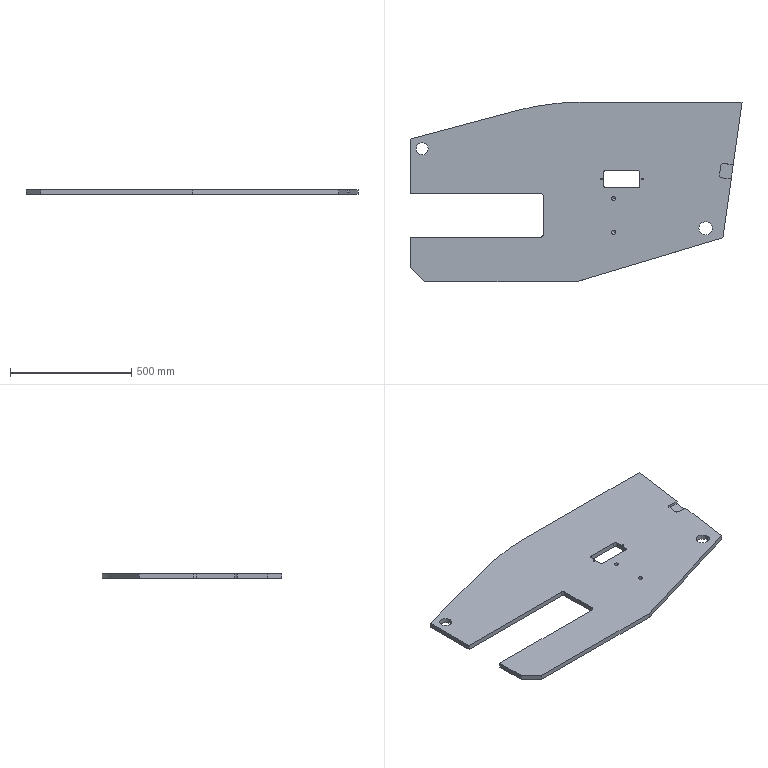Part | SolidWorks | features HoleWzd 2, FlatPattern 1, ICE 1, SMBaseFlange 1, SheetMetal 1 | 1 solid | 50 faces | box 1372 x 742.1 x 20 mm | volume 15301514 mm3 | cylinder 21 | plane 21 | cone 8 | commonest cylinder face diameters 20 x8 6.8 x4 17.5 x4 50 x2 55 x2 2000 x1
STEP:
#1=CARTESIAN_POINT('',(833.25,344.5,-12.));
#2=VERTEX_POINT('',#1);
#3=CARTESIAN_POINT('',(850.75,344.5,-12.));
#4=VERTEX_POINT('',#3);
#5=CARTESIAN_POINT('',(842.,344.5,-12.));
#6=DIRECTION('',(0.,0.,1.));
#7=DIRECTION('',(1.,0.,0.));
#8=AXIS2_PLACEMENT_3D('',#5,#6,#7);
#9=CIRCLE('',#8,8.75);
#10=EDGE_CURVE('',#2,#4,#9,.T.);
#11=ORIENTED_EDGE('',*,*,#10,.F.);
#12=CARTESIAN_POINT('',(833.25,344.5,0.));
#13=VERTEX_POINT('',#12);
#14=CARTESIAN_POINT('',(833.25,344.5,0.));
#15=DIRECTION('',(0.,0.,1.));
#16=VECTOR('',#15,1000.);
#17=LINE('',#14,#16);
#18=EDGE_CURVE('',#2,#13,#17,.T.);
#19=ORIENTED_EDGE('',*,*,#18,.T.);
#20=CARTESIAN_POINT('',(850.75,344.5,0.));
#21=VERTEX_POINT('',#20);
#22=CARTESIAN_POINT('',(842.,344.5,0.));
#23=DIRECTION('',(0.,0.,1.));
#24=DIRECTION('',(1.,0.,0.));
#25=AXIS2_PLACEMENT_3D('',#22,#23,#24);
#26=CIRCLE('',#25,8.75);
#27=EDGE_CURVE('',#13,#21,#26,.T.);
#28=ORIENTED_EDGE('',*,*,#27,.T.);
#29=CARTESIAN_POINT('',(850.75,344.5,0.));
#30=DIRECTION('',(0.,0.,1.));
#31=VECTOR('',#30,1000.);
#32=LINE('',#29,#31);
#33=EDGE_CURVE('',#4,#21,#32,.T.);
#34=ORIENTED_EDGE('',*,*,#33,.F.);
#35=EDGE_LOOP('',(#11,#19,#28,#34));
#36=FACE_OUTER_BOUND('',#35,.T.);
#37=CARTESIAN_POINT('',(842.,344.5,0.));
#38=DIRECTION('',(0.,0.,1.));
#39=DIRECTION('',(1.,0.,0.));
#40=AXIS2_PLACEMENT_3D('',#37,#38,#39);
#41=CYLINDRICAL_SURFACE('',#40,8.75);
#42=ADVANCED_FACE('',(#36),#41,.F.);
#43=CARTESIAN_POINT('',(842.,344.5,-17.258));
#44=VERTEX_POINT('',#43);
#45=CARTESIAN_POINT('',(850.75,344.5,-12.));
#46=DIRECTION('',(0.8572,0.,0.515));
#47=VECTOR('',#46,1000.);
#48=LINE('',#45,#47);
#49=EDGE_CURVE('',#44,#4,#48,.T.);
#50=ORIENTED_EDGE('',*,*,#49,.F.);
#51=CARTESIAN_POINT('',(833.25,344.5,-12.));
#52=DIRECTION('',(-0.8572,0.,0.515));
#53=VECTOR('',#52,1000.);
#54=LINE('',#51,#53);
#55=EDGE_CURVE('',#44,#2,#54,.T.);
#56=ORIENTED_EDGE('',*,*,#55,.T.);
#57=ORIENTED_EDGE('',*,*,#10,.T.);
#58=EDGE_LOOP('',(#50,#56,#57));
#59=FACE_OUTER_BOUND('',#58,.T.);
#60=CARTESIAN_POINT('',(842.,344.5,-12.));
#61=DIRECTION('',(0.,0.,1.));
#62=DIRECTION('',(1.,0.,0.));
#63=AXIS2_PLACEMENT_3D('',#60,#61,#62);
#64=CONICAL_SURFACE('',#63,8.75,1.03);
#65=ADVANCED_FACE('',(#59),#64,.F.);
#66=CARTESIAN_POINT('',(833.25,204.5,-12.));
#67=VERTEX_POINT('',#66);
#68=CARTESIAN_POINT('',(850.75,204.5,-12.));
#69=VERTEX_POINT('',#68);
#70=CARTESIAN_POINT('',(842.,204.5,-12.));
#71=DIRECTION('',(0.,0.,1.));
#72=DIRECTION('',(1.,0.,0.));
#73=AXIS2_PLACEMENT_3D('',#70,#71,#72);
#74=CIRCLE('',#73,8.75);
#75=EDGE_CURVE('',#67,#69,#74,.T.);
#76=ORIENTED_EDGE('',*,*,#75,.F.);
#77=CARTESIAN_POINT('',(833.25,204.5,0.));
#78=VERTEX_POINT('',#77);
#79=CARTESIAN_POINT('',(833.25,204.5,0.));
#80=DIRECTION('',(0.,0.,1.));
#81=VECTOR('',#80,1000.);
#82=LINE('',#79,#81);
#83=EDGE_CURVE('',#67,#78,#82,.T.);
#84=ORIENTED_EDGE('',*,*,#83,.T.);
#85=CARTESIAN_POINT('',(850.75,204.5,0.));
#86=VERTEX_POINT('',#85);
#87=CARTESIAN_POINT('',(842.,204.5,0.));
#88=DIRECTION('',(0.,0.,1.));
#89=DIRECTION('',(1.,0.,0.));
#90=AXIS2_PLACEMENT_3D('',#87,#88,#89);
#91=CIRCLE('',#90,8.75);
#92=EDGE_CURVE('',#78,#86,#91,.T.);
#93=ORIENTED_EDGE('',*,*,#92,.T.);
#94=CARTESIAN_POINT('',(850.75,204.5,0.));
#95=DIRECTION('',(0.,0.,1.));
#96=VECTOR('',#95,1000.);
#97=LINE('',#94,#96);
#98=EDGE_CURVE('',#69,#86,#97,.T.);
#99=ORIENTED_EDGE('',*,*,#98,.F.);
#100=EDGE_LOOP('',(#76,#84,#93,#99));
#101=FACE_OUTER_BOUND('',#100,.T.);
#102=CARTESIAN_POINT('',(842.,204.5,0.));
#103=DIRECTION('',(0.,0.,1.));
#104=DIRECTION('',(1.,0.,0.));
#105=AXIS2_PLACEMENT_3D('',#102,#103,#104);
#106=CYLINDRICAL_SURFACE('',#105,8.75);
#107=ADVANCED_FACE('',(#101),#106,.F.);
#108=CARTESIAN_POINT('',(842.,204.5,-17.258));
#109=VERTEX_POINT('',#108);
#110=CARTESIAN_POINT('',(850.75,204.5,-12.));
#111=DIRECTION('',(0.8572,0.,0.515));
#112=VECTOR('',#111,1000.);
#113=LINE('',#110,#112);
#114=EDGE_CURVE('',#109,#69,#113,.T.);
#115=ORIENTED_EDGE('',*,*,#114,.F.);
#116=CARTESIAN_POINT('',(833.25,204.5,-12.));
#117=DIRECTION('',(-0.8572,0.,0.515));
#118=VECTOR('',#117,1000.);
#119=LINE('',#116,#118);
#120=EDGE_CURVE('',#109,#67,#119,.T.);
#121=ORIENTED_EDGE('',*,*,#120,.T.);
#122=ORIENTED_EDGE('',*,*,#75,.T.);
#123=EDGE_LOOP('',(#115,#121,#122));
#124=FACE_OUTER_BOUND('',#123,.T.);
#125=CARTESIAN_POINT('',(842.,204.5,-12.));
#126=DIRECTION('',(0.,0.,1.));
#127=DIRECTION('',(1.,0.,0.));
#128=AXIS2_PLACEMENT_3D('',#125,#126,#127);
#129=CONICAL_SURFACE('',#128,8.75,1.03);
#130=ADVANCED_FACE('',(#124),#129,.F.);
#131=CARTESIAN_POINT('',(786.6,424.5,-12.));
#132=VERTEX_POINT('',#131);
#133=CARTESIAN_POINT('',(793.4,424.5,-12.));
#134=VERTEX_POINT('',#133);
#135=CARTESIAN_POINT('',(790.,424.5,-12.));
#136=DIRECTION('',(0.,0.,1.));
#137=DIRECTION('',(1.,0.,0.));
#138=AXIS2_PLACEMENT_3D('',#135,#136,#137);
#139=CIRCLE('',#138,3.4);
#140=EDGE_CURVE('',#132,#134,#139,.T.);
#141=ORIENTED_EDGE('',*,*,#140,.F.);
#142=CARTESIAN_POINT('',(786.6,424.5,0.));
#143=VERTEX_POINT('',#142);
#144=CARTESIAN_POINT('',(786.6,424.5,0.));
#145=DIRECTION('',(0.,0.,1.));
#146=VECTOR('',#145,1000.);
#147=LINE('',#144,#146);
#148=EDGE_CURVE('',#132,#143,#147,.T.);
#149=ORIENTED_EDGE('',*,*,#148,.T.);
#150=CARTESIAN_POINT('',(793.4,424.5,0.));
#151=VERTEX_POINT('',#150);
#152=CARTESIAN_POINT('',(790.,424.5,0.));
#153=DIRECTION('',(0.,0.,1.));
#154=DIRECTION('',(1.,0.,0.));
#155=AXIS2_PLACEMENT_3D('',#152,#153,#154);
#156=CIRCLE('',#155,3.4);
#157=EDGE_CURVE('',#143,#151,#156,.T.);
#158=ORIENTED_EDGE('',*,*,#157,.T.);
#159=CARTESIAN_POINT('',(793.4,424.5,0.));
#160=DIRECTION('',(0.,0.,1.));
#161=VECTOR('',#160,1000.);
#162=LINE('',#159,#161);
#163=EDGE_CURVE('',#134,#151,#162,.T.);
#164=ORIENTED_EDGE('',*,*,#163,.F.);
#165=EDGE_LOOP('',(#141,#149,#158,#164));
#166=FACE_OUTER_BOUND('',#165,.T.);
#167=CARTESIAN_POINT('',(790.,424.5,0.));
#168=DIRECTION('',(0.,0.,1.));
#169=DIRECTION('',(1.,0.,0.));
#170=AXIS2_PLACEMENT_3D('',#167,#168,#169);
#171=CYLINDRICAL_SURFACE('',#170,3.4);
#172=ADVANCED_FACE('',(#166),#171,.F.);
#173=CARTESIAN_POINT('',(790.,424.5,-14.043));
#174=VERTEX_POINT('',#173);
#175=CARTESIAN_POINT('',(793.4,424.5,-12.));
#176=DIRECTION('',(0.8572,0.,0.515));
#177=VECTOR('',#176,1000.);
#178=LINE('',#175,#177);
#179=EDGE_CURVE('',#174,#134,#178,.T.);
#180=ORIENTED_EDGE('',*,*,#179,.F.);
#181=CARTESIAN_POINT('',(786.6,424.5,-12.));
#182=DIRECTION('',(-0.8572,0.,0.515));
#183=VECTOR('',#182,1000.);
#184=LINE('',#181,#183);
#185=EDGE_CURVE('',#174,#132,#184,.T.);
#186=ORIENTED_EDGE('',*,*,#185,.T.);
#187=ORIENTED_EDGE('',*,*,#140,.T.);
#188=EDGE_LOOP('',(#180,#186,#187));
#189=FACE_OUTER_BOUND('',#188,.T.);
#190=CARTESIAN_POINT('',(790.,424.5,-12.));
#191=DIRECTION('',(0.,0.,1.));
#192=DIRECTION('',(1.,0.,0.));
#193=AXIS2_PLACEMENT_3D('',#190,#191,#192);
#194=CONICAL_SURFACE('',#193,3.4,1.03);
#195=ADVANCED_FACE('',(#189),#194,.F.);
#196=CARTESIAN_POINT('',(956.6,424.5,-12.));
#197=VERTEX_POINT('',#196);
#198=CARTESIAN_POINT('',(963.4,424.5,-12.));
#199=VERTEX_POINT('',#198);
#200=CARTESIAN_POINT('',(960.,424.5,-12.));
#201=DIRECTION('',(0.,0.,1.));
#202=DIRECTION('',(1.,0.,0.));
#203=AXIS2_PLACEMENT_3D('',#200,#201,#202);
#204=CIRCLE('',#203,3.4);
#205=EDGE_CURVE('',#197,#199,#204,.T.);
#206=ORIENTED_EDGE('',*,*,#205,.F.);
#207=CARTESIAN_POINT('',(956.6,424.5,0.));
#208=VERTEX_POINT('',#207);
#209=CARTESIAN_POINT('',(956.6,424.5,0.));
#210=DIRECTION('',(0.,0.,1.));
#211=VECTOR('',#210,1000.);
#212=LINE('',#209,#211);
#213=EDGE_CURVE('',#197,#208,#212,.T.);
#214=ORIENTED_EDGE('',*,*,#213,.T.);
#215=CARTESIAN_POINT('',(963.4,424.5,0.));
#216=VERTEX_POINT('',#215);
#217=CARTESIAN_POINT('',(960.,424.5,0.));
#218=DIRECTION('',(0.,0.,1.));
#219=DIRECTION('',(1.,0.,0.));
#220=AXIS2_PLACEMENT_3D('',#217,#218,#219);
#221=CIRCLE('',#220,3.4);
#222=EDGE_CURVE('',#208,#216,#221,.T.);
#223=ORIENTED_EDGE('',*,*,#222,.T.);
#224=CARTESIAN_POINT('',(963.4,424.5,0.));
#225=DIRECTION('',(0.,0.,1.));
#226=VECTOR('',#225,1000.);
#227=LINE('',#224,#226);
#228=EDGE_CURVE('',#199,#216,#227,.T.);
#229=ORIENTED_EDGE('',*,*,#228,.F.);
#230=EDGE_LOOP('',(#206,#214,#223,#229));
#231=FACE_OUTER_BOUND('',#230,.T.);
#232=CARTESIAN_POINT('',(960.,424.5,0.));
#233=DIRECTION('',(0.,0.,1.));
#234=DIRECTION('',(1.,0.,0.));
#235=AXIS2_PLACEMENT_3D('',#232,#233,#234);
#236=CYLINDRICAL_SURFACE('',#235,3.4);
#237=ADVANCED_FACE('',(#231),#236,.F.);
#238=CARTESIAN_POINT('',(960.,424.5,-14.043));
#239=VERTEX_POINT('',#238);
#240=CARTESIAN_POINT('',(963.4,424.5,-12.));
#241=DIRECTION('',(0.8572,0.,0.515));
#242=VECTOR('',#241,1000.);
#243=LINE('',#240,#242);
#244=EDGE_CURVE('',#239,#199,#243,.T.);
#245=ORIENTED_EDGE('',*,*,#244,.F.);
#246=CARTESIAN_POINT('',(956.6,424.5,-12.));
#247=DIRECTION('',(-0.8572,0.,0.515));
#248=VECTOR('',#247,1000.);
#249=LINE('',#246,#248);
#250=EDGE_CURVE('',#239,#197,#249,.T.);
#251=ORIENTED_EDGE('',*,*,#250,.T.);
#252=ORIENTED_EDGE('',*,*,#205,.T.);
#253=EDGE_LOOP('',(#245,#251,#252));
#254=FACE_OUTER_BOUND('',#253,.T.);
#255=CARTESIAN_POINT('',(960.,424.5,-12.));
#256=DIRECTION('',(0.,0.,1.));
#257=DIRECTION('',(1.,0.,0.));
#258=AXIS2_PLACEMENT_3D('',#255,#256,#257);
#259=CONICAL_SURFACE('',#258,3.4,1.03);
#260=ADVANCED_FACE('',(#254),#259,.F.);
#261=CARTESIAN_POINT('',(1194.,220.7,-20.));
#262=VERTEX_POINT('',#261);
#263=CARTESIAN_POINT('',(1249.,220.7,-20.));
#264=VERTEX_POINT('',#263);
#265=CARTESIAN_POINT('',(1221.5,220.7,-20.));
#266=DIRECTION('',(0.,0.,1.));
#267=DIRECTION('',(1.,0.,0.));
#268=AXIS2_PLACEMENT_3D('',#265,#266,#267);
#269=CIRCLE('',#268,27.5);
#270=EDGE_CURVE('',#262,#264,#269,.T.);
#271=ORIENTED_EDGE('',*,*,#270,.F.);
#272=CARTESIAN_POINT('',(1194.,220.7,0.));
#273=VERTEX_POINT('',#272);
#274=CARTESIAN_POINT('',(1194.,220.7,-20.));
#275=DIRECTION('',(0.,0.,1.));
#276=VECTOR('',#275,1000.);
#277=LINE('',#274,#276);
#278=EDGE_CURVE('',#262,#273,#277,.T.);
#279=ORIENTED_EDGE('',*,*,#278,.T.);
#280=CARTESIAN_POINT('',(1249.,220.7,0.));
#281=VERTEX_POINT('',#280);
#282=CARTESIAN_POINT('',(1221.5,220.7,0.));
#283=DIRECTION('',(0.,0.,1.));
#284=DIRECTION('',(1.,0.,0.));
#285=AXIS2_PLACEMENT_3D('',#282,#283,#284);
#286=CIRCLE('',#285,27.5);
#287=EDGE_CURVE('',#273,#281,#286,.T.);
#288=ORIENTED_EDGE('',*,*,#287,.T.);
#289=CARTESIAN_POINT('',(1249.,220.7,-20.));
#290=DIRECTION('',(0.,0.,1.));
#291=VECTOR('',#290,1000.);
#292=LINE('',#289,#291);
#293=EDGE_CURVE('',#264,#281,#292,.T.);
#294=ORIENTED_EDGE('',*,*,#293,.F.);
#295=EDGE_LOOP('',(#271,#279,#288,#294));
#296=FACE_OUTER_BOUND('',#295,.T.);
#297=CARTESIAN_POINT('',(1221.5,220.7,-20.));
#298=DIRECTION('',(0.,0.,1.));
#299=DIRECTION('',(1.,0.,0.));
#300=AXIS2_PLACEMENT_3D('',#297,#298,#299);
#301=CYLINDRICAL_SURFACE('',#300,27.5);
#302=ADVANCED_FACE('',(#296),#301,.F.);
#303=CARTESIAN_POINT('',(25.,550.,-20.));
#304=VERTEX_POINT('',#303);
#305=CARTESIAN_POINT('',(75.,550.,-20.));
#306=VERTEX_POINT('',#305);
#307=CARTESIAN_POINT('',(50.,550.,-20.));
#308=DIRECTION('',(0.,0.,1.));
#309=DIRECTION('',(1.,0.,0.));
#310=AXIS2_PLACEMENT_3D('',#307,#308,#309);
#311=CIRCLE('',#310,25.);
#312=EDGE_CURVE('',#304,#306,#311,.T.);
#313=ORIENTED_EDGE('',*,*,#312,.F.);
#314=CARTESIAN_POINT('',(25.,550.,0.));
#315=VERTEX_POINT('',#314);
#316=CARTESIAN_POINT('',(25.,550.,-20.));
#317=DIRECTION('',(0.,0.,1.));
#318=VECTOR('',#317,1000.);
#319=LINE('',#316,#318);
#320=EDGE_CURVE('',#304,#315,#319,.T.);
#321=ORIENTED_EDGE('',*,*,#320,.T.);
#322=CARTESIAN_POINT('',(75.,550.,0.));
#323=VERTEX_POINT('',#322);
#324=CARTESIAN_POINT('',(50.,550.,0.));
#325=DIRECTION('',(0.,0.,1.));
#326=DIRECTION('',(1.,0.,0.));
#327=AXIS2_PLACEMENT_3D('',#324,#325,#326);
#328=CIRCLE('',#327,25.);
#329=EDGE_CURVE('',#315,#323,#328,.T.);
#330=ORIENTED_EDGE('',*,*,#329,.T.);
#331=CARTESIAN_POINT('',(75.,550.,-20.));
#332=DIRECTION('',(0.,0.,1.));
#333=VECTOR('',#332,1000.);
#334=LINE('',#331,#333);
#335=EDGE_CURVE('',#306,#323,#334,.T.);
#336=ORIENTED_EDGE('',*,*,#335,.F.);
#337=EDGE_LOOP('',(#313,#321,#330,#336));
#338=FACE_OUTER_BOUND('',#337,.T.);
#339=CARTESIAN_POINT('',(50.,550.,-20.));
#340=DIRECTION('',(0.,0.,1.));
#341=DIRECTION('',(1.,0.,0.));
#342=AXIS2_PLACEMENT_3D('',#339,#340,#341);
#343=CYLINDRICAL_SURFACE('',#342,25.);
#344=ADVANCED_FACE('',(#338),#343,.F.);
#345=CARTESIAN_POINT('',(0.,590.,0.));
#346=VERTEX_POINT('',#345);
#347=CARTESIAN_POINT('',(0.,364.5,0.));
#348=VERTEX_POINT('',#347);
#349=CARTESIAN_POINT('',(0.,364.5,0.));
#350=DIRECTION('',(0.,-1.,0.));
#351=VECTOR('',#350,1000.);
#352=LINE('',#349,#351);
#353=EDGE_CURVE('',#346,#348,#352,.T.);
#354=ORIENTED_EDGE('',*,*,#353,.F.);
#355=CARTESIAN_POINT('',(0.,590.,-20.));
#356=VERTEX_POINT('',#355);
#357=CARTESIAN_POINT('',(0.,590.,-20.));
#358=DIRECTION('',(0.,0.,1.));
#359=VECTOR('',#358,1000.);
#360=LINE('',#357,#359);
#361=EDGE_CURVE('',#356,#346,#360,.T.);
#362=ORIENTED_EDGE('',*,*,#361,.F.);
#363=CARTESIAN_POINT('',(0.,364.5,-20.));
#364=VERTEX_POINT('',#363);
#365=CARTESIAN_POINT('',(0.,364.5,-20.));
#366=DIRECTION('',(0.,-1.,0.));
#367=VECTOR('',#366,1000.);
#368=LINE('',#365,#367);
#369=EDGE_CURVE('',#356,#364,#368,.T.);
#370=ORIENTED_EDGE('',*,*,#369,.T.);
#371=CARTESIAN_POINT('',(0.,364.5,-20.));
#372=DIRECTION('',(0.,0.,1.));
#373=VECTOR('',#372,1000.);
#374=LINE('',#371,#373);
#375=EDGE_CURVE('',#364,#348,#374,.T.);
#376=ORIENTED_EDGE('',*,*,#375,.T.);
#377=EDGE_LOOP('',(#354,#362,#370,#376));
#378=FACE_OUTER_BOUND('',#377,.T.);
#379=CARTESIAN_POINT('',(0.,364.5,-20.));
#380=DIRECTION('',(-1.,0.,0.));
#381=DIRECTION('',(0.,0.,1.));
#382=AXIS2_PLACEMENT_3D('',#379,#380,#381);
#383=PLANE('',#382);
#384=ADVANCED_FACE('',(#378),#383,.T.);
#385=CARTESIAN_POINT('',(445.345,708.483,0.));
#386=VERTEX_POINT('',#385);
#387=CARTESIAN_POINT('',(0.,590.,0.));
#388=DIRECTION('',(-0.9664,-0.2571,0.));
#389=VECTOR('',#388,1000.);
#390=LINE('',#387,#389);
#391=EDGE_CURVE('',#386,#346,#390,.T.);
#392=ORIENTED_EDGE('',*,*,#391,.F.);
#393=CARTESIAN_POINT('',(445.345,708.483,-20.));
#394=VERTEX_POINT('',#393);
#395=CARTESIAN_POINT('',(445.345,708.483,-20.));
#396=DIRECTION('',(0.,0.,1.));
#397=VECTOR('',#396,1000.);
#398=LINE('',#395,#397);
#399=EDGE_CURVE('',#394,#386,#398,.T.);
#400=ORIENTED_EDGE('',*,*,#399,.F.);
#401=CARTESIAN_POINT('',(0.,590.,-20.));
#402=DIRECTION('',(-0.9664,-0.2571,0.));
#403=VECTOR('',#402,1000.);
#404=LINE('',#401,#403);
#405=EDGE_CURVE('',#394,#356,#404,.T.);
#406=ORIENTED_EDGE('',*,*,#405,.T.);
#407=ORIENTED_EDGE('',*,*,#361,.T.);
#408=EDGE_LOOP('',(#392,#400,#406,#407));
#409=FACE_OUTER_BOUND('',#408,.T.);
#410=CARTESIAN_POINT('',(0.,590.,-20.));
#411=DIRECTION('',(-0.2571,0.9664,0.));
#412=DIRECTION('',(-0.9664,-0.2571,0.));
#413=AXIS2_PLACEMENT_3D('',#410,#411,#412);
#414=PLANE('',#413);
#415=ADVANCED_FACE('',(#409),#414,.T.);
#416=CARTESIAN_POINT('',(702.45,742.1,0.));
#417=VERTEX_POINT('',#416);
#418=CARTESIAN_POINT('',(702.45,-257.9,0.));
#419=DIRECTION('',(0.,0.,1.));
#420=DIRECTION('',(1.,0.,0.));
#421=AXIS2_PLACEMENT_3D('',#418,#419,#420);
#422=CIRCLE('',#421,1000.);
#423=EDGE_CURVE('',#417,#386,#422,.T.);
#424=ORIENTED_EDGE('',*,*,#423,.F.);
#425=CARTESIAN_POINT('',(702.45,742.1,-20.));
#426=VERTEX_POINT('',#425);
#427=CARTESIAN_POINT('',(702.45,742.1,-20.));
#428=DIRECTION('',(0.,0.,1.));
#429=VECTOR('',#428,1000.);
#430=LINE('',#427,#429);
#431=EDGE_CURVE('',#426,#417,#430,.T.);
#432=ORIENTED_EDGE('',*,*,#431,.F.);
#433=CARTESIAN_POINT('',(702.45,-257.9,-20.));
#434=DIRECTION('',(0.,0.,1.));
#435=DIRECTION('',(1.,0.,0.));
#436=AXIS2_PLACEMENT_3D('',#433,#434,#435);
#437=CIRCLE('',#436,1000.);
#438=EDGE_CURVE('',#426,#394,#437,.T.);
#439=ORIENTED_EDGE('',*,*,#438,.T.);
#440=ORIENTED_EDGE('',*,*,#399,.T.);
#441=EDGE_LOOP('',(#424,#432,#439,#440));
#442=FACE_OUTER_BOUND('',#441,.T.);
#443=CARTESIAN_POINT('',(702.45,-257.9,-20.));
#444=DIRECTION('',(0.,0.,1.));
#445=DIRECTION('',(1.,0.,0.));
#446=AXIS2_PLACEMENT_3D('',#443,#444,#445);
#447=CYLINDRICAL_SURFACE('',#446,1000.);
#448=ADVANCED_FACE('',(#442),#447,.T.);
#449=CARTESIAN_POINT('',(1371.7,742.1,0.));
#450=VERTEX_POINT('',#449);
#451=CARTESIAN_POINT('',(702.45,742.1,0.));
#452=DIRECTION('',(-1.,0.,0.));
#453=VECTOR('',#452,1000.);
#454=LINE('',#451,#453);
#455=EDGE_CURVE('',#450,#417,#454,.T.);
#456=ORIENTED_EDGE('',*,*,#455,.F.);
#457=CARTESIAN_POINT('',(1371.7,742.1,-20.));
#458=VERTEX_POINT('',#457);
#459=CARTESIAN_POINT('',(1371.7,742.1,-20.));
#460=DIRECTION('',(0.,0.,1.));
#461=VECTOR('',#460,1000.);
#462=LINE('',#459,#461);
#463=EDGE_CURVE('',#458,#450,#462,.T.);
#464=ORIENTED_EDGE('',*,*,#463,.F.);
#465=CARTESIAN_POINT('',(702.45,742.1,-20.));
#466=DIRECTION('',(-1.,0.,0.));
#467=VECTOR('',#466,1000.);
#468=LINE('',#465,#467);
#469=EDGE_CURVE('',#458,#426,#468,.T.);
#470=ORIENTED_EDGE('',*,*,#469,.T.);
#471=ORIENTED_EDGE('',*,*,#431,.T.);
#472=EDGE_LOOP('',(#456,#464,#470,#471));
#473=FACE_OUTER_BOUND('',#472,.T.);
#474=CARTESIAN_POINT('',(702.45,742.1,-20.));
#475=DIRECTION('',(0.,1.,0.));
#476=DIRECTION('',(0.,0.,1.));
#477=AXIS2_PLACEMENT_3D('',#474,#475,#476);
#478=PLANE('',#477);
#479=ADVANCED_FACE('',(#473),#478,.T.);
#480=CARTESIAN_POINT('',(1327.066,424.218,-10.));
#481=VERTEX_POINT('',#480);
#482=CARTESIAN_POINT('',(1327.066,424.218,0.));
#483=VERTEX_POINT('',#482);
#484=CARTESIAN_POINT('',(1327.066,424.218,-10.));
#485=DIRECTION('',(0.,0.,1.));
#486=VECTOR('',#485,1000.);
#487=LINE('',#484,#486);
#488=EDGE_CURVE('',#481,#483,#487,.T.);
#489=ORIENTED_EDGE('',*,*,#488,.T.);
#490=CARTESIAN_POINT('',(1293.,181.6,0.));
#491=VERTEX_POINT('',#490);
#492=CARTESIAN_POINT('',(1371.7,742.1,0.));
#493=DIRECTION('',(0.139,0.9903,0.));
#494=VECTOR('',#493,1000.);
#495=LINE('',#492,#494);
#496=EDGE_CURVE('',#491,#483,#495,.T.);
#497=ORIENTED_EDGE('',*,*,#496,.F.);
#498=CARTESIAN_POINT('',(1293.,181.6,-20.));
#499=VERTEX_POINT('',#498);
#500=CARTESIAN_POINT('',(1293.,181.6,-20.));
#501=DIRECTION('',(0.,0.,1.));
#502=VECTOR('',#501,1000.);
#503=LINE('',#500,#502);
#504=EDGE_CURVE('',#499,#491,#503,.T.);
#505=ORIENTED_EDGE('',*,*,#504,.F.);
#506=CARTESIAN_POINT('',(1371.7,742.1,-20.));
#507=DIRECTION('',(0.139,0.9903,0.));
#508=VECTOR('',#507,1000.);
#509=LINE('',#506,#508);
#510=EDGE_CURVE('',#499,#458,#509,.T.);
#511=ORIENTED_EDGE('',*,*,#510,.T.);
#512=ORIENTED_EDGE('',*,*,#463,.T.);
#513=CARTESIAN_POINT('',(1335.409,483.635,0.));
#514=VERTEX_POINT('',#513);
#515=CARTESIAN_POINT('',(1371.7,742.1,0.));
#516=DIRECTION('',(0.139,0.9903,0.));
#517=VECTOR('',#516,1000.);
#518=LINE('',#515,#517);
#519=EDGE_CURVE('',#514,#450,#518,.T.);
#520=ORIENTED_EDGE('',*,*,#519,.F.);
#521=CARTESIAN_POINT('',(1335.409,483.635,-10.));
#522=VERTEX_POINT('',#521);
#523=CARTESIAN_POINT('',(1335.409,483.635,-10.));
#524=DIRECTION('',(0.,0.,1.));
#525=VECTOR('',#524,1000.);
#526=LINE('',#523,#525);
#527=EDGE_CURVE('',#522,#514,#526,.T.);
#528=ORIENTED_EDGE('',*,*,#527,.F.);
#529=CARTESIAN_POINT('',(1327.066,424.218,-10.));
#530=DIRECTION('',(0.139,0.9903,0.));
#531=VECTOR('',#530,1000.);
#532=LINE('',#529,#531);
#533=EDGE_CURVE('',#481,#522,#532,.T.);
#534=ORIENTED_EDGE('',*,*,#533,.F.);
#535=EDGE_LOOP('',(#489,#497,#505,#511,#512,#520,#528,#534));
#536=FACE_OUTER_BOUND('',#535,.T.);
#537=CARTESIAN_POINT('',(1371.7,742.1,-20.));
#538=DIRECTION('',(0.9903,-0.139,0.));
#539=DIRECTION('',(0.139,0.9903,0.));
#540=AXIS2_PLACEMENT_3D('',#537,#538,#539);
#541=PLANE('',#540);
#542=ADVANCED_FACE('',(#536),#541,.T.);
#543=CARTESIAN_POINT('',(688.,0.,0.));
#544=VERTEX_POINT('',#543);
#545=CARTESIAN_POINT('',(688.,0.,0.));
#546=DIRECTION('',(0.9578,0.2875,0.));
#547=VECTOR('',#546,1000.);
#548=LINE('',#545,#547);
#549=EDGE_CURVE('',#544,#491,#548,.T.);
#550=ORIENTED_EDGE('',*,*,#549,.F.);
#551=CARTESIAN_POINT('',(688.,0.,-20.));
#552=VERTEX_POINT('',#551);
#553=CARTESIAN_POINT('',(688.,0.,-20.));
#554=DIRECTION('',(0.,0.,1.));
#555=VECTOR('',#554,1000.);
#556=LINE('',#553,#555);
#557=EDGE_CURVE('',#552,#544,#556,.T.);
#558=ORIENTED_EDGE('',*,*,#557,.F.);
#559=CARTESIAN_POINT('',(688.,0.,-20.));
#560=DIRECTION('',(0.9578,0.2875,0.));
#561=VECTOR('',#560,1000.);
#562=LINE('',#559,#561);
#563=EDGE_CURVE('',#552,#499,#562,.T.);
#564=ORIENTED_EDGE('',*,*,#563,.T.);
#565=ORIENTED_EDGE('',*,*,#504,.T.);
#566=EDGE_LOOP('',(#550,#558,#564,#565));
#567=FACE_OUTER_BOUND('',#566,.T.);
#568=CARTESIAN_POINT('',(688.,0.,-20.));
#569=DIRECTION('',(0.2875,-0.9578,0.));
#570=DIRECTION('',(0.9578,0.2875,0.));
#571=AXIS2_PLACEMENT_3D('',#568,#569,#570);
#572=PLANE('',#571);
#573=ADVANCED_FACE('',(#567),#572,.T.);
#574=CARTESIAN_POINT('',(60.,0.,0.));
#575=VERTEX_POINT('',#574);
#576=CARTESIAN_POINT('',(688.,0.,0.));
#577=DIRECTION('',(1.,0.,0.));
#578=VECTOR('',#577,1000.);
#579=LINE('',#576,#578);
#580=EDGE_CURVE('',#575,#544,#579,.T.);
#581=ORIENTED_EDGE('',*,*,#580,.F.);
#582=CARTESIAN_POINT('',(60.,0.,-20.));
#583=VERTEX_POINT('',#582);
#584=CARTESIAN_POINT('',(60.,0.,-20.));
#585=DIRECTION('',(0.,0.,1.));
#586=VECTOR('',#585,1000.);
#587=LINE('',#584,#586);
#588=EDGE_CURVE('',#583,#575,#587,.T.);
#589=ORIENTED_EDGE('',*,*,#588,.F.);
#590=CARTESIAN_POINT('',(688.,0.,-20.));
#591=DIRECTION('',(1.,0.,0.));
#592=VECTOR('',#591,1000.);
#593=LINE('',#590,#592);
#594=EDGE_CURVE('',#583,#552,#593,.T.);
#595=ORIENTED_EDGE('',*,*,#594,.T.);
#596=ORIENTED_EDGE('',*,*,#557,.T.);
#597=EDGE_LOOP('',(#581,#589,#595,#596));
#598=FACE_OUTER_BOUND('',#597,.T.);
#599=CARTESIAN_POINT('',(688.,0.,-20.));
#600=DIRECTION('',(0.,-1.,0.));
#601=DIRECTION('',(0.,0.,-1.));
#602=AXIS2_PLACEMENT_3D('',#599,#600,#601);
#603=PLANE('',#602);
#604=ADVANCED_FACE('',(#598),#603,.T.);
#605=CARTESIAN_POINT('',(0.,60.,0.));
#606=VERTEX_POINT('',#605);
#607=CARTESIAN_POINT('',(60.,0.,0.));
#608=DIRECTION('',(0.7071,-0.7071,0.));
#609=VECTOR('',#608,1000.);
#610=LINE('',#607,#609);
#611=EDGE_CURVE('',#606,#575,#610,.T.);
#612=ORIENTED_EDGE('',*,*,#611,.F.);
#613=CARTESIAN_POINT('',(0.,60.,-20.));
#614=VERTEX_POINT('',#613);
#615=CARTESIAN_POINT('',(0.,60.,-20.));
#616=DIRECTION('',(0.,0.,1.));
#617=VECTOR('',#616,1000.);
#618=LINE('',#615,#617);
#619=EDGE_CURVE('',#614,#606,#618,.T.);
#620=ORIENTED_EDGE('',*,*,#619,.F.);
#621=CARTESIAN_POINT('',(60.,0.,-20.));
#622=DIRECTION('',(0.7071,-0.7071,0.));
#623=VECTOR('',#622,1000.);
#624=LINE('',#621,#623);
#625=EDGE_CURVE('',#614,#583,#624,.T.);
#626=ORIENTED_EDGE('',*,*,#625,.T.);
#627=ORIENTED_EDGE('',*,*,#588,.T.);
#628=EDGE_LOOP('',(#612,#620,#626,#627));
#629=FACE_OUTER_BOUND('',#628,.T.);
#630=CARTESIAN_POINT('',(60.,0.,-20.));
#631=DIRECTION('',(-0.7071,-0.7071,0.));
#632=DIRECTION('',(0.7071,-0.7071,0.));
#633=AXIS2_PLACEMENT_3D('',#630,#631,#632);
#634=PLANE('',#633);
#635=ADVANCED_FACE('',(#629),#634,.T.);
#636=CARTESIAN_POINT('',(0.,184.5,0.));
#637=VERTEX_POINT('',#636);
#638=CARTESIAN_POINT('',(0.,60.,0.));
#639=DIRECTION('',(0.,-1.,0.));
#640=VECTOR('',#639,1000.);
#641=LINE('',#638,#640);
#642=EDGE_CURVE('',#637,#606,#641,.T.);
#643=ORIENTED_EDGE('',*,*,#642,.F.);
#644=CARTESIAN_POINT('',(0.,184.5,-20.));
#645=VERTEX_POINT('',#644);
#646=CARTESIAN_POINT('',(0.,184.5,-20.));
#647=DIRECTION('',(0.,0.,1.));
#648=VECTOR('',#647,1000.);
#649=LINE('',#646,#648);
#650=EDGE_CURVE('',#645,#637,#649,.T.);
#651=ORIENTED_EDGE('',*,*,#650,.F.);
#652=CARTESIAN_POINT('',(0.,60.,-20.));
#653=DIRECTION('',(0.,-1.,0.));
#654=VECTOR('',#653,1000.);
#655=LINE('',#652,#654);
#656=EDGE_CURVE('',#645,#614,#655,.T.);
#657=ORIENTED_EDGE('',*,*,#656,.T.);
#658=ORIENTED_EDGE('',*,*,#619,.T.);
#659=EDGE_LOOP('',(#643,#651,#657,#658));
#660=FACE_OUTER_BOUND('',#659,.T.);
#661=CARTESIAN_POINT('',(0.,60.,-20.));
#662=DIRECTION('',(-1.,0.,0.));
#663=DIRECTION('',(0.,-1.,0.));
#664=AXIS2_PLACEMENT_3D('',#661,#662,#663);
#665=PLANE('',#664);
#666=ADVANCED_FACE('',(#660),#665,.T.);
#667=CARTESIAN_POINT('',(540.,184.5,0.));
#668=VERTEX_POINT('',#667);
#669=CARTESIAN_POINT('',(540.,184.5,0.));
#670=DIRECTION('',(-1.,0.,0.));
#671=VECTOR('',#670,1000.);
#672=LINE('',#669,#671);
#673=EDGE_CURVE('',#668,#637,#672,.T.);
#674=ORIENTED_EDGE('',*,*,#673,.F.);
#675=CARTESIAN_POINT('',(540.,184.5,-20.));
#676=VERTEX_POINT('',#675);
#677=CARTESIAN_POINT('',(540.,184.5,-20.));
#678=DIRECTION('',(0.,0.,1.));
#679=VECTOR('',#678,1000.);
#680=LINE('',#677,#679);
#681=EDGE_CURVE('',#676,#668,#680,.T.);
#682=ORIENTED_EDGE('',*,*,#681,.F.);
#683=CARTESIAN_POINT('',(540.,184.5,-20.));
#684=DIRECTION('',(-1.,0.,0.));
#685=VECTOR('',#684,1000.);
#686=LINE('',#683,#685);
#687=EDGE_CURVE('',#676,#645,#686,.T.);
#688=ORIENTED_EDGE('',*,*,#687,.T.);
#689=ORIENTED_EDGE('',*,*,#650,.T.);
#690=EDGE_LOOP('',(#674,#682,#688,#689));
#691=FACE_OUTER_BOUND('',#690,.T.);
#692=CARTESIAN_POINT('',(540.,184.5,-20.));
#693=DIRECTION('',(0.,1.,0.));
#694=DIRECTION('',(-1.,0.,0.));
#695=AXIS2_PLACEMENT_3D('',#692,#693,#694);
#696=PLANE('',#695);
#697=ADVANCED_FACE('',(#691),#696,.T.);
#698=CARTESIAN_POINT('',(550.,194.5,0.));
#699=VERTEX_POINT('',#698);
#700=CARTESIAN_POINT('',(540.,194.5,0.));
#701=DIRECTION('',(0.,0.,-1.));
#702=DIRECTION('',(1.,0.,0.));
#703=AXIS2_PLACEMENT_3D('',#700,#701,#702);
#704=CIRCLE('',#703,10.);
#705=EDGE_CURVE('',#699,#668,#704,.T.);
#706=ORIENTED_EDGE('',*,*,#705,.F.);
#707=CARTESIAN_POINT('',(550.,194.5,-20.));
#708=VERTEX_POINT('',#707);
#709=CARTESIAN_POINT('',(550.,194.5,-20.));
#710=DIRECTION('',(0.,0.,1.));
#711=VECTOR('',#710,1000.);
#712=LINE('',#709,#711);
#713=EDGE_CURVE('',#708,#699,#712,.T.);
#714=ORIENTED_EDGE('',*,*,#713,.F.);
#715=CARTESIAN_POINT('',(540.,194.5,-20.));
#716=DIRECTION('',(0.,0.,-1.));
#717=DIRECTION('',(1.,0.,0.));
#718=AXIS2_PLACEMENT_3D('',#715,#716,#717);
#719=CIRCLE('',#718,10.);
#720=EDGE_CURVE('',#708,#676,#719,.T.);
#721=ORIENTED_EDGE('',*,*,#720,.T.);
#722=ORIENTED_EDGE('',*,*,#681,.T.);
#723=EDGE_LOOP('',(#706,#714,#721,#722));
#724=FACE_OUTER_BOUND('',#723,.T.);
#725=CARTESIAN_POINT('',(540.,194.5,-20.));
#726=DIRECTION('',(0.,0.,1.));
#727=DIRECTION('',(1.,0.,0.));
#728=AXIS2_PLACEMENT_3D('',#725,#726,#727);
#729=CYLINDRICAL_SURFACE('',#728,10.);
#730=ADVANCED_FACE('',(#724),#729,.F.);
#731=CARTESIAN_POINT('',(550.,354.5,0.));
#732=VERTEX_POINT('',#731);
#733=CARTESIAN_POINT('',(550.,354.5,0.));
#734=DIRECTION('',(0.,-1.,0.));
#735=VECTOR('',#734,1000.);
#736=LINE('',#733,#735);
#737=EDGE_CURVE('',#732,#699,#736,.T.);
#738=ORIENTED_EDGE('',*,*,#737,.F.);
#739=CARTESIAN_POINT('',(550.,354.5,-20.));
#740=VERTEX_POINT('',#739);
#741=CARTESIAN_POINT('',(550.,354.5,-20.));
#742=DIRECTION('',(0.,0.,1.));
#743=VECTOR('',#742,1000.);
#744=LINE('',#741,#743);
#745=EDGE_CURVE('',#740,#732,#744,.T.);
#746=ORIENTED_EDGE('',*,*,#745,.F.);
#747=CARTESIAN_POINT('',(550.,354.5,-20.));
#748=DIRECTION('',(0.,-1.,0.));
#749=VECTOR('',#748,1000.);
#750=LINE('',#747,#749);
#751=EDGE_CURVE('',#740,#708,#750,.T.);
#752=ORIENTED_EDGE('',*,*,#751,.T.);
#753=ORIENTED_EDGE('',*,*,#713,.T.);
#754=EDGE_LOOP('',(#738,#746,#752,#753));
#755=FACE_OUTER_BOUND('',#754,.T.);
#756=CARTESIAN_POINT('',(550.,354.5,-20.));
#757=DIRECTION('',(-1.,0.,0.));
#758=DIRECTION('',(0.,0.,1.));
#759=AXIS2_PLACEMENT_3D('',#756,#757,#758);
#760=PLANE('',#759);
#761=ADVANCED_FACE('',(#755),#760,.T.);
#762=CARTESIAN_POINT('',(540.,364.5,0.));
#763=VERTEX_POINT('',#762);
#764=CARTESIAN_POINT('',(540.,354.5,0.));
#765=DIRECTION('',(0.,0.,-1.));
#766=DIRECTION('',(1.,0.,0.));
#767=AXIS2_PLACEMENT_3D('',#764,#765,#766);
#768=CIRCLE('',#767,10.);
#769=EDGE_CURVE('',#763,#732,#768,.T.);
#770=ORIENTED_EDGE('',*,*,#769,.F.);
#771=CARTESIAN_POINT('',(540.,364.5,-20.));
#772=VERTEX_POINT('',#771);
#773=CARTESIAN_POINT('',(540.,364.5,-20.));
#774=DIRECTION('',(0.,0.,1.));
#775=VECTOR('',#774,1000.);
#776=LINE('',#773,#775);
#777=EDGE_CURVE('',#772,#763,#776,.T.);
#778=ORIENTED_EDGE('',*,*,#777,.F.);
#779=CARTESIAN_POINT('',(540.,354.5,-20.));
#780=DIRECTION('',(0.,0.,-1.));
#781=DIRECTION('',(1.,0.,0.));
#782=AXIS2_PLACEMENT_3D('',#779,#780,#781);
#783=CIRCLE('',#782,10.);
#784=EDGE_CURVE('',#772,#740,#783,.T.);
#785=ORIENTED_EDGE('',*,*,#784,.T.);
#786=ORIENTED_EDGE('',*,*,#745,.T.);
#787=EDGE_LOOP('',(#770,#778,#785,#786));
#788=FACE_OUTER_BOUND('',#787,.T.);
#789=CARTESIAN_POINT('',(540.,354.5,-20.));
#790=DIRECTION('',(0.,0.,1.));
#791=DIRECTION('',(1.,0.,0.));
#792=AXIS2_PLACEMENT_3D('',#789,#790,#791);
#793=CYLINDRICAL_SURFACE('',#792,10.);
#794=ADVANCED_FACE('',(#788),#793,.F.);
#795=CARTESIAN_POINT('',(0.,364.5,0.));
#796=DIRECTION('',(1.,0.,0.));
#797=VECTOR('',#796,1000.);
#798=LINE('',#795,#797);
#799=EDGE_CURVE('',#348,#763,#798,.T.);
#800=ORIENTED_EDGE('',*,*,#799,.F.);
#801=ORIENTED_EDGE('',*,*,#375,.F.);
#802=CARTESIAN_POINT('',(0.,364.5,-20.));
#803=DIRECTION('',(1.,0.,0.));
#804=VECTOR('',#803,1000.);
#805=LINE('',#802,#804);
#806=EDGE_CURVE('',#364,#772,#805,.T.);
#807=ORIENTED_EDGE('',*,*,#806,.T.);
#808=ORIENTED_EDGE('',*,*,#777,.T.);
#809=EDGE_LOOP('',(#800,#801,#807,#808));
#810=FACE_OUTER_BOUND('',#809,.T.);
#811=CARTESIAN_POINT('',(0.,364.5,-20.));
#812=DIRECTION('',(0.,-1.,0.));
#813=DIRECTION('',(1.,0.,0.));
#814=AXIS2_PLACEMENT_3D('',#811,#812,#813);
#815=PLANE('',#814);
#816=ADVANCED_FACE('',(#810),#815,.T.);
#817=CARTESIAN_POINT('',(1221.5,220.7,-20.));
#818=DIRECTION('',(0.,0.,1.));
#819=DIRECTION('',(1.,0.,0.));
#820=AXIS2_PLACEMENT_3D('',#817,#818,#819);
#821=CIRCLE('',#820,27.5);
#822=EDGE_CURVE('',#264,#262,#821,.T.);
#823=ORIENTED_EDGE('',*,*,#822,.T.);
#824=ORIENTED_EDGE('',*,*,#270,.T.);
#825=EDGE_LOOP('',(#823,#824));
#826=FACE_BOUND('',#825,.T.);
#827=CARTESIAN_POINT('',(50.,550.,-20.));
#828=DIRECTION('',(0.,0.,1.));
#829=DIRECTION('',(1.,0.,0.));
#830=AXIS2_PLACEMENT_3D('',#827,#828,#829);
#831=CIRCLE('',#830,25.);
#832=EDGE_CURVE('',#306,#304,#831,.T.);
#833=ORIENTED_EDGE('',*,*,#832,.T.);
#834=ORIENTED_EDGE('',*,*,#312,.T.);
#835=EDGE_LOOP('',(#833,#834));
#836=FACE_BOUND('',#835,.T.);
#837=CARTESIAN_POINT('',(810.,389.5,-20.));
#838=VERTEX_POINT('',#837);
#839=CARTESIAN_POINT('',(940.,389.5,-20.));
#840=VERTEX_POINT('',#839);
#841=CARTESIAN_POINT('',(810.,389.5,-20.));
#842=DIRECTION('',(1.,0.,0.));
#843=VECTOR('',#842,1000.);
#844=LINE('',#841,#843);
#845=EDGE_CURVE('',#838,#840,#844,.T.);
#846=ORIENTED_EDGE('',*,*,#845,.T.);
#847=CARTESIAN_POINT('',(950.,399.5,-20.));
#848=VERTEX_POINT('',#847);
#849=CARTESIAN_POINT('',(940.,399.5,-20.));
#850=DIRECTION('',(0.,0.,1.));
#851=DIRECTION('',(1.,0.,0.));
#852=AXIS2_PLACEMENT_3D('',#849,#850,#851);
#853=CIRCLE('',#852,10.);
#854=EDGE_CURVE('',#840,#848,#853,.T.);
#855=ORIENTED_EDGE('',*,*,#854,.T.);
#856=CARTESIAN_POINT('',(950.,449.5,-20.));
#857=VERTEX_POINT('',#856);
#858=CARTESIAN_POINT('',(950.,449.5,-20.));
#859=DIRECTION('',(0.,1.,0.));
#860=VECTOR('',#859,1000.);
#861=LINE('',#858,#860);
#862=EDGE_CURVE('',#848,#857,#861,.T.);
#863=ORIENTED_EDGE('',*,*,#862,.T.);
#864=CARTESIAN_POINT('',(940.,459.5,-20.));
#865=VERTEX_POINT('',#864);
#866=CARTESIAN_POINT('',(940.,449.5,-20.));
#867=DIRECTION('',(0.,0.,1.));
#868=DIRECTION('',(1.,0.,0.));
#869=AXIS2_PLACEMENT_3D('',#866,#867,#868);
#870=CIRCLE('',#869,10.);
#871=EDGE_CURVE('',#857,#865,#870,.T.);
#872=ORIENTED_EDGE('',*,*,#871,.T.);
#873=CARTESIAN_POINT('',(810.,459.5,-20.));
#874=VERTEX_POINT('',#873);
#875=CARTESIAN_POINT('',(810.,459.5,-20.));
#876=DIRECTION('',(-1.,0.,0.));
#877=VECTOR('',#876,1000.);
#878=LINE('',#875,#877);
#879=EDGE_CURVE('',#865,#874,#878,.T.);
#880=ORIENTED_EDGE('',*,*,#879,.T.);
#881=CARTESIAN_POINT('',(800.,449.5,-20.));
#882=VERTEX_POINT('',#881);
#883=CARTESIAN_POINT('',(810.,449.5,-20.));
#884=DIRECTION('',(0.,0.,1.));
#885=DIRECTION('',(1.,0.,0.));
#886=AXIS2_PLACEMENT_3D('',#883,#884,#885);
#887=CIRCLE('',#886,10.);
#888=EDGE_CURVE('',#874,#882,#887,.T.);
#889=ORIENTED_EDGE('',*,*,#888,.T.);
#890=CARTESIAN_POINT('',(800.,399.5,-20.));
#891=VERTEX_POINT('',#890);
#892=CARTESIAN_POINT('',(800.,449.5,-20.));
#893=DIRECTION('',(0.,-1.,0.));
#894=VECTOR('',#893,1000.);
#895=LINE('',#892,#894);
#896=EDGE_CURVE('',#882,#891,#895,.T.);
#897=ORIENTED_EDGE('',*,*,#896,.T.);
#898=CARTESIAN_POINT('',(810.,399.5,-20.));
#899=DIRECTION('',(0.,0.,1.));
#900=DIRECTION('',(-1.,0.,0.));
#901=AXIS2_PLACEMENT_3D('',#898,#899,#900);
#902=CIRCLE('',#901,10.);
#903=EDGE_CURVE('',#891,#838,#902,.T.);
#904=ORIENTED_EDGE('',*,*,#903,.T.);
#905=EDGE_LOOP('',(#846,#855,#863,#872,#880,#889,#897,#904));
#906=FACE_BOUND('',#905,.T.);
#907=ORIENTED_EDGE('',*,*,#369,.F.);
#908=ORIENTED_EDGE('',*,*,#405,.F.);
#909=ORIENTED_EDGE('',*,*,#438,.F.);
#910=ORIENTED_EDGE('',*,*,#469,.F.);
#911=ORIENTED_EDGE('',*,*,#510,.F.);
#912=ORIENTED_EDGE('',*,*,#563,.F.);
#913=ORIENTED_EDGE('',*,*,#594,.F.);
#914=ORIENTED_EDGE('',*,*,#625,.F.);
#915=ORIENTED_EDGE('',*,*,#656,.F.);
#916=ORIENTED_EDGE('',*,*,#687,.F.);
#917=ORIENTED_EDGE('',*,*,#720,.F.);
#918=ORIENTED_EDGE('',*,*,#751,.F.);
#919=ORIENTED_EDGE('',*,*,#784,.F.);
#920=ORIENTED_EDGE('',*,*,#806,.F.);
#921=EDGE_LOOP('',(#907,#908,#909,#910,#911,#912,#913,#914,#915,#916,#917,#918,#919,#920));
#922=FACE_OUTER_BOUND('',#921,.T.);
#923=CARTESIAN_POINT('',(702.45,-257.9,-20.));
#924=DIRECTION('',(0.,0.,1.));
#925=DIRECTION('',(1.,0.,0.));
#926=AXIS2_PLACEMENT_3D('',#923,#924,#925);
#927=PLANE('',#926);
#928=ADVANCED_FACE('',(#826,#836,#906,#922),#927,.F.);
#929=CARTESIAN_POINT('',(1287.455,429.78,0.));
#930=VERTEX_POINT('',#929);
#931=CARTESIAN_POINT('',(1287.455,429.78,0.));
#932=DIRECTION('',(0.9903,-0.139,0.));
#933=VECTOR('',#932,1000.);
#934=LINE('',#931,#933);
#935=EDGE_CURVE('',#930,#483,#934,.T.);
#936=ORIENTED_EDGE('',*,*,#935,.F.);
#937=CARTESIAN_POINT('',(1278.942,441.073,0.));
#938=VERTEX_POINT('',#937);
#939=CARTESIAN_POINT('',(1288.845,439.683,0.));
#940=DIRECTION('',(0.,0.,1.));
#941=DIRECTION('',(-1.,0.,0.));
#942=AXIS2_PLACEMENT_3D('',#939,#940,#941);
#943=CIRCLE('',#942,10.);
#944=EDGE_CURVE('',#938,#930,#943,.T.);
#945=ORIENTED_EDGE('',*,*,#944,.F.);
#946=CARTESIAN_POINT('',(1284.504,480.685,0.));
#947=VERTEX_POINT('',#946);
#948=CARTESIAN_POINT('',(1284.504,480.685,0.));
#949=DIRECTION('',(-0.139,-0.9903,0.));
#950=VECTOR('',#949,1000.);
#951=LINE('',#948,#950);
#952=EDGE_CURVE('',#947,#938,#951,.T.);
#953=ORIENTED_EDGE('',*,*,#952,.F.);
#954=CARTESIAN_POINT('',(1295.797,489.197,0.));
#955=VERTEX_POINT('',#954);
#956=CARTESIAN_POINT('',(1294.407,479.294,0.));
#957=DIRECTION('',(0.,0.,1.));
#958=DIRECTION('',(-1.,0.,0.));
#959=AXIS2_PLACEMENT_3D('',#956,#957,#958);
#960=CIRCLE('',#959,10.);
#961=EDGE_CURVE('',#955,#947,#960,.T.);
#962=ORIENTED_EDGE('',*,*,#961,.F.);
#963=CARTESIAN_POINT('',(1335.409,483.635,0.));
#964=DIRECTION('',(-0.9903,0.139,0.));
#965=VECTOR('',#964,1000.);
#966=LINE('',#963,#965);
#967=EDGE_CURVE('',#514,#955,#966,.T.);
#968=ORIENTED_EDGE('',*,*,#967,.F.);
#969=ORIENTED_EDGE('',*,*,#519,.T.);
#970=ORIENTED_EDGE('',*,*,#455,.T.);
#971=ORIENTED_EDGE('',*,*,#423,.T.);
#972=ORIENTED_EDGE('',*,*,#391,.T.);
#973=ORIENTED_EDGE('',*,*,#353,.T.);
#974=ORIENTED_EDGE('',*,*,#799,.T.);
#975=ORIENTED_EDGE('',*,*,#769,.T.);
#976=ORIENTED_EDGE('',*,*,#737,.T.);
#977=ORIENTED_EDGE('',*,*,#705,.T.);
#978=ORIENTED_EDGE('',*,*,#673,.T.);
#979=ORIENTED_EDGE('',*,*,#642,.T.);
#980=ORIENTED_EDGE('',*,*,#611,.T.);
#981=ORIENTED_EDGE('',*,*,#580,.T.);
#982=ORIENTED_EDGE('',*,*,#549,.T.);
#983=ORIENTED_EDGE('',*,*,#496,.T.);
#984=EDGE_LOOP('',(#936,#945,#953,#962,#968,#969,#970,#971,#972,#973,#974,#975,#976,#977,#978,#979,#980,#981,#982,#983));
#985=FACE_OUTER_BOUND('',#984,.T.);
#986=CARTESIAN_POINT('',(842.,344.5,0.));
#987=DIRECTION('',(0.,0.,1.));
#988=DIRECTION('',(1.,0.,0.));
#989=AXIS2_PLACEMENT_3D('',#986,#987,#988);
#990=CIRCLE('',#989,8.75);
#991=EDGE_CURVE('',#21,#13,#990,.T.);
#992=ORIENTED_EDGE('',*,*,#991,.F.);
#993=ORIENTED_EDGE('',*,*,#27,.F.);
#994=EDGE_LOOP('',(#992,#993));
#995=FACE_BOUND('',#994,.T.);
#996=CARTESIAN_POINT('',(842.,204.5,0.));
#997=DIRECTION('',(0.,0.,1.));
#998=DIRECTION('',(1.,0.,0.));
#999=AXIS2_PLACEMENT_3D('',#996,#997,#998);
#1000=CIRCLE('',#999,8.75);
#1001=EDGE_CURVE('',#86,#78,#1000,.T.);
#1002=ORIENTED_EDGE('',*,*,#1001,.F.);
#1003=ORIENTED_EDGE('',*,*,#92,.F.);
#1004=EDGE_LOOP('',(#1002,#1003));
#1005=FACE_BOUND('',#1004,.T.);
#1006=CARTESIAN_POINT('',(790.,424.5,0.));
#1007=DIRECTION('',(0.,0.,1.));
#1008=DIRECTION('',(1.,0.,0.));
#1009=AXIS2_PLACEMENT_3D('',#1006,#1007,#1008);
#1010=CIRCLE('',#1009,3.4);
#1011=EDGE_CURVE('',#151,#143,#1010,.T.);
#1012=ORIENTED_EDGE('',*,*,#1011,.F.);
#1013=ORIENTED_EDGE('',*,*,#157,.F.);
#1014=EDGE_LOOP('',(#1012,#1013));
#1015=FACE_BOUND('',#1014,.T.);
#1016=CARTESIAN_POINT('',(960.,424.5,0.));
#1017=DIRECTION('',(0.,0.,1.));
#1018=DIRECTION('',(1.,0.,0.));
#1019=AXIS2_PLACEMENT_3D('',#1016,#1017,#1018);
#1020=CIRCLE('',#1019,3.4);
#1021=EDGE_CURVE('',#216,#208,#1020,.T.);
#1022=ORIENTED_EDGE('',*,*,#1021,.F.);
#1023=ORIENTED_EDGE('',*,*,#222,.F.);
#1024=EDGE_LOOP('',(#1022,#1023));
#1025=FACE_BOUND('',#1024,.T.);
#1026=CARTESIAN_POINT('',(1221.5,220.7,0.));
#1027=DIRECTION('',(0.,0.,1.));
#1028=DIRECTION('',(1.,0.,0.));
#1029=AXIS2_PLACEMENT_3D('',#1026,#1027,#1028);
#1030=CIRCLE('',#1029,27.5);
#1031=EDGE_CURVE('',#281,#273,#1030,.T.);
#1032=ORIENTED_EDGE('',*,*,#1031,.F.);
#1033=ORIENTED_EDGE('',*,*,#287,.F.);
#1034=EDGE_LOOP('',(#1032,#1033));
#1035=FACE_BOUND('',#1034,.T.);
#1036=CARTESIAN_POINT('',(50.,550.,0.));
#1037=DIRECTION('',(0.,0.,1.));
#1038=DIRECTION('',(1.,0.,0.));
#1039=AXIS2_PLACEMENT_3D('',#1036,#1037,#1038);
#1040=CIRCLE('',#1039,25.);
#1041=EDGE_CURVE('',#323,#315,#1040,.T.);
#1042=ORIENTED_EDGE('',*,*,#1041,.F.);
#1043=ORIENTED_EDGE('',*,*,#329,.F.);
#1044=EDGE_LOOP('',(#1042,#1043));
#1045=FACE_BOUND('',#1044,.T.);
#1046=CARTESIAN_POINT('',(940.,389.5,0.));
#1047=VERTEX_POINT('',#1046);
#1048=CARTESIAN_POINT('',(950.,399.5,0.));
#1049=VERTEX_POINT('',#1048);
#1050=CARTESIAN_POINT('',(940.,399.5,0.));
#1051=DIRECTION('',(0.,0.,1.));
#1052=DIRECTION('',(1.,0.,0.));
#1053=AXIS2_PLACEMENT_3D('',#1050,#1051,#1052);
#1054=CIRCLE('',#1053,10.);
#1055=EDGE_CURVE('',#1047,#1049,#1054,.T.);
#1056=ORIENTED_EDGE('',*,*,#1055,.F.);
#1057=CARTESIAN_POINT('',(810.,389.5,0.));
#1058=VERTEX_POINT('',#1057);
#1059=CARTESIAN_POINT('',(810.,389.5,0.));
#1060=DIRECTION('',(1.,0.,0.));
#1061=VECTOR('',#1060,1000.);
#1062=LINE('',#1059,#1061);
#1063=EDGE_CURVE('',#1058,#1047,#1062,.T.);
#1064=ORIENTED_EDGE('',*,*,#1063,.F.);
#1065=CARTESIAN_POINT('',(800.,399.5,0.));
#1066=VERTEX_POINT('',#1065);
#1067=CARTESIAN_POINT('',(810.,399.5,0.));
#1068=DIRECTION('',(0.,0.,1.));
#1069=DIRECTION('',(-1.,0.,0.));
#1070=AXIS2_PLACEMENT_3D('',#1067,#1068,#1069);
#1071=CIRCLE('',#1070,10.);
#1072=EDGE_CURVE('',#1066,#1058,#1071,.T.);
#1073=ORIENTED_EDGE('',*,*,#1072,.F.);
#1074=CARTESIAN_POINT('',(800.,449.5,0.));
#1075=VERTEX_POINT('',#1074);
#1076=CARTESIAN_POINT('',(800.,449.5,0.));
#1077=DIRECTION('',(0.,-1.,0.));
#1078=VECTOR('',#1077,1000.);
#1079=LINE('',#1076,#1078);
#1080=EDGE_CURVE('',#1075,#1066,#1079,.T.);
#1081=ORIENTED_EDGE('',*,*,#1080,.F.);
#1082=CARTESIAN_POINT('',(810.,459.5,0.));
#1083=VERTEX_POINT('',#1082);
#1084=CARTESIAN_POINT('',(810.,449.5,0.));
#1085=DIRECTION('',(0.,0.,1.));
#1086=DIRECTION('',(1.,0.,0.));
#1087=AXIS2_PLACEMENT_3D('',#1084,#1085,#1086);
#1088=CIRCLE('',#1087,10.);
#1089=EDGE_CURVE('',#1083,#1075,#1088,.T.);
#1090=ORIENTED_EDGE('',*,*,#1089,.F.);
#1091=CARTESIAN_POINT('',(940.,459.5,0.));
#1092=VERTEX_POINT('',#1091);
#1093=CARTESIAN_POINT('',(810.,459.5,0.));
#1094=DIRECTION('',(-1.,0.,0.));
#1095=VECTOR('',#1094,1000.);
#1096=LINE('',#1093,#1095);
#1097=EDGE_CURVE('',#1092,#1083,#1096,.T.);
#1098=ORIENTED_EDGE('',*,*,#1097,.F.);
#1099=CARTESIAN_POINT('',(950.,449.5,0.));
#1100=VERTEX_POINT('',#1099);
#1101=CARTESIAN_POINT('',(940.,449.5,0.));
#1102=DIRECTION('',(0.,0.,1.));
#1103=DIRECTION('',(1.,0.,0.));
#1104=AXIS2_PLACEMENT_3D('',#1101,#1102,#1103);
#1105=CIRCLE('',#1104,10.);
#1106=EDGE_CURVE('',#1100,#1092,#1105,.T.);
#1107=ORIENTED_EDGE('',*,*,#1106,.F.);
#1108=CARTESIAN_POINT('',(950.,449.5,0.));
#1109=DIRECTION('',(0.,1.,0.));
#1110=VECTOR('',#1109,1000.);
#1111=LINE('',#1108,#1110);
#1112=EDGE_CURVE('',#1049,#1100,#1111,.T.);
#1113=ORIENTED_EDGE('',*,*,#1112,.F.);
#1114=EDGE_LOOP('',(#1056,#1064,#1073,#1081,#1090,#1098,#1107,#1113));
#1115=FACE_BOUND('',#1114,.T.);
#1116=CARTESIAN_POINT('',(702.45,-257.9,0.));
#1117=DIRECTION('',(0.,0.,1.));
#1118=DIRECTION('',(1.,0.,0.));
#1119=AXIS2_PLACEMENT_3D('',#1116,#1117,#1118);
#1120=PLANE('',#1119);
#1121=ADVANCED_FACE('',(#985,#995,#1005,#1015,#1025,#1035,#1045,#1115),#1120,.T.);
#1122=ORIENTED_EDGE('',*,*,#1055,.T.);
#1123=CARTESIAN_POINT('',(950.,399.5,-20.));
#1124=DIRECTION('',(0.,0.,1.));
#1125=VECTOR('',#1124,1000.);
#1126=LINE('',#1123,#1125);
#1127=EDGE_CURVE('',#848,#1049,#1126,.T.);
#1128=ORIENTED_EDGE('',*,*,#1127,.F.);
#1129=ORIENTED_EDGE('',*,*,#854,.F.);
#1130=CARTESIAN_POINT('',(940.,389.5,-20.));
#1131=DIRECTION('',(0.,0.,1.));
#1132=VECTOR('',#1131,1000.);
#1133=LINE('',#1130,#1132);
#1134=EDGE_CURVE('',#840,#1047,#1133,.T.);
#1135=ORIENTED_EDGE('',*,*,#1134,.T.);
#1136=EDGE_LOOP('',(#1122,#1128,#1129,#1135));
#1137=FACE_OUTER_BOUND('',#1136,.T.);
#1138=CARTESIAN_POINT('',(940.,399.5,-20.));
#1139=DIRECTION('',(0.,0.,1.));
#1140=DIRECTION('',(1.,0.,0.));
#1141=AXIS2_PLACEMENT_3D('',#1138,#1139,#1140);
#1142=CYLINDRICAL_SURFACE('',#1141,10.);
#1143=ADVANCED_FACE('',(#1137),#1142,.F.);
#1144=ORIENTED_EDGE('',*,*,#1063,.T.);
#1145=ORIENTED_EDGE('',*,*,#1134,.F.);
#1146=ORIENTED_EDGE('',*,*,#845,.F.);
#1147=CARTESIAN_POINT('',(810.,389.5,-20.));
#1148=DIRECTION('',(0.,0.,1.));
#1149=VECTOR('',#1148,1000.);
#1150=LINE('',#1147,#1149);
#1151=EDGE_CURVE('',#838,#1058,#1150,.T.);
#1152=ORIENTED_EDGE('',*,*,#1151,.T.);
#1153=EDGE_LOOP('',(#1144,#1145,#1146,#1152));
#1154=FACE_OUTER_BOUND('',#1153,.T.);
#1155=CARTESIAN_POINT('',(810.,389.5,-20.));
#1156=DIRECTION('',(0.,-1.,0.));
#1157=DIRECTION('',(1.,0.,0.));
#1158=AXIS2_PLACEMENT_3D('',#1155,#1156,#1157);
#1159=PLANE('',#1158);
#1160=ADVANCED_FACE('',(#1154),#1159,.F.);
#1161=ORIENTED_EDGE('',*,*,#1072,.T.);
#1162=ORIENTED_EDGE('',*,*,#1151,.F.);
#1163=ORIENTED_EDGE('',*,*,#903,.F.);
#1164=CARTESIAN_POINT('',(800.,399.5,-20.));
#1165=DIRECTION('',(0.,0.,1.));
#1166=VECTOR('',#1165,1000.);
#1167=LINE('',#1164,#1166);
#1168=EDGE_CURVE('',#891,#1066,#1167,.T.);
#1169=ORIENTED_EDGE('',*,*,#1168,.T.);
#1170=EDGE_LOOP('',(#1161,#1162,#1163,#1169));
#1171=FACE_OUTER_BOUND('',#1170,.T.);
#1172=CARTESIAN_POINT('',(810.,399.5,-20.));
#1173=DIRECTION('',(0.,0.,1.));
#1174=DIRECTION('',(1.,0.,0.));
#1175=AXIS2_PLACEMENT_3D('',#1172,#1173,#1174);
#1176=CYLINDRICAL_SURFACE('',#1175,10.);
#1177=ADVANCED_FACE('',(#1171),#1176,.F.);
#1178=ORIENTED_EDGE('',*,*,#1080,.T.);
#1179=ORIENTED_EDGE('',*,*,#1168,.F.);
#1180=ORIENTED_EDGE('',*,*,#896,.F.);
#1181=CARTESIAN_POINT('',(800.,449.5,-20.));
#1182=DIRECTION('',(0.,0.,1.));
#1183=VECTOR('',#1182,1000.);
#1184=LINE('',#1181,#1183);
#1185=EDGE_CURVE('',#882,#1075,#1184,.T.);
#1186=ORIENTED_EDGE('',*,*,#1185,.T.);
#1187=EDGE_LOOP('',(#1178,#1179,#1180,#1186));
#1188=FACE_OUTER_BOUND('',#1187,.T.);
#1189=CARTESIAN_POINT('',(800.,449.5,-20.));
#1190=DIRECTION('',(-1.,0.,0.));
#1191=DIRECTION('',(0.,0.,1.));
#1192=AXIS2_PLACEMENT_3D('',#1189,#1190,#1191);
#1193=PLANE('',#1192);
#1194=ADVANCED_FACE('',(#1188),#1193,.F.);
#1195=ORIENTED_EDGE('',*,*,#1089,.T.);
#1196=ORIENTED_EDGE('',*,*,#1185,.F.);
#1197=ORIENTED_EDGE('',*,*,#888,.F.);
#1198=CARTESIAN_POINT('',(810.,459.5,-20.));
#1199=DIRECTION('',(0.,0.,1.));
#1200=VECTOR('',#1199,1000.);
#1201=LINE('',#1198,#1200);
#1202=EDGE_CURVE('',#874,#1083,#1201,.T.);
#1203=ORIENTED_EDGE('',*,*,#1202,.T.);
#1204=EDGE_LOOP('',(#1195,#1196,#1197,#1203));
#1205=FACE_OUTER_BOUND('',#1204,.T.);
#1206=CARTESIAN_POINT('',(810.,449.5,-20.));
#1207=DIRECTION('',(0.,0.,1.));
#1208=DIRECTION('',(1.,0.,0.));
#1209=AXIS2_PLACEMENT_3D('',#1206,#1207,#1208);
#1210=CYLINDRICAL_SURFACE('',#1209,10.);
#1211=ADVANCED_FACE('',(#1205),#1210,.F.);
#1212=ORIENTED_EDGE('',*,*,#1097,.T.);
#1213=ORIENTED_EDGE('',*,*,#1202,.F.);
#1214=ORIENTED_EDGE('',*,*,#879,.F.);
#1215=CARTESIAN_POINT('',(940.,459.5,-20.));
#1216=DIRECTION('',(0.,0.,1.));
#1217=VECTOR('',#1216,1000.);
#1218=LINE('',#1215,#1217);
#1219=EDGE_CURVE('',#865,#1092,#1218,.T.);
#1220=ORIENTED_EDGE('',*,*,#1219,.T.);
#1221=EDGE_LOOP('',(#1212,#1213,#1214,#1220));
#1222=FACE_OUTER_BOUND('',#1221,.T.);
#1223=CARTESIAN_POINT('',(810.,459.5,-20.));
#1224=DIRECTION('',(0.,1.,0.));
#1225=DIRECTION('',(0.,0.,1.));
#1226=AXIS2_PLACEMENT_3D('',#1223,#1224,#1225);
#1227=PLANE('',#1226);
#1228=ADVANCED_FACE('',(#1222),#1227,.F.);
#1229=ORIENTED_EDGE('',*,*,#1106,.T.);
#1230=ORIENTED_EDGE('',*,*,#1219,.F.);
#1231=ORIENTED_EDGE('',*,*,#871,.F.);
#1232=CARTESIAN_POINT('',(950.,449.5,-20.));
#1233=DIRECTION('',(0.,0.,1.));
#1234=VECTOR('',#1233,1000.);
#1235=LINE('',#1232,#1234);
#1236=EDGE_CURVE('',#857,#1100,#1235,.T.);
#1237=ORIENTED_EDGE('',*,*,#1236,.T.);
#1238=EDGE_LOOP('',(#1229,#1230,#1231,#1237));
#1239=FACE_OUTER_BOUND('',#1238,.T.);
#1240=CARTESIAN_POINT('',(940.,449.5,-20.));
#1241=DIRECTION('',(0.,0.,1.));
#1242=DIRECTION('',(1.,0.,0.));
#1243=AXIS2_PLACEMENT_3D('',#1240,#1241,#1242);
#1244=CYLINDRICAL_SURFACE('',#1243,10.);
#1245=ADVANCED_FACE('',(#1239),#1244,.F.);
#1246=ORIENTED_EDGE('',*,*,#1112,.T.);
#1247=ORIENTED_EDGE('',*,*,#1236,.F.);
#1248=ORIENTED_EDGE('',*,*,#862,.F.);
#1249=ORIENTED_EDGE('',*,*,#1127,.T.);
#1250=EDGE_LOOP('',(#1246,#1247,#1248,#1249));
#1251=FACE_OUTER_BOUND('',#1250,.T.);
#1252=CARTESIAN_POINT('',(950.,449.5,-20.));
#1253=DIRECTION('',(1.,0.,0.));
#1254=DIRECTION('',(0.,0.,-1.));
#1255=AXIS2_PLACEMENT_3D('',#1252,#1253,#1254);
#1256=PLANE('',#1255);
#1257=ADVANCED_FACE('',(#1251),#1256,.F.);
#1258=ORIENTED_EDGE('',*,*,#320,.F.);
#1259=ORIENTED_EDGE('',*,*,#832,.F.);
#1260=ORIENTED_EDGE('',*,*,#335,.T.);
#1261=ORIENTED_EDGE('',*,*,#1041,.T.);
#1262=EDGE_LOOP('',(#1258,#1259,#1260,#1261));
#1263=FACE_OUTER_BOUND('',#1262,.T.);
#1264=CARTESIAN_POINT('',(50.,550.,-20.));
#1265=DIRECTION('',(0.,0.,1.));
#1266=DIRECTION('',(1.,0.,0.));
#1267=AXIS2_PLACEMENT_3D('',#1264,#1265,#1266);
#1268=CYLINDRICAL_SURFACE('',#1267,25.);
#1269=ADVANCED_FACE('',(#1263),#1268,.F.);
#1270=ORIENTED_EDGE('',*,*,#278,.F.);
#1271=ORIENTED_EDGE('',*,*,#822,.F.);
#1272=ORIENTED_EDGE('',*,*,#293,.T.);
#1273=ORIENTED_EDGE('',*,*,#1031,.T.);
#1274=EDGE_LOOP('',(#1270,#1271,#1272,#1273));
#1275=FACE_OUTER_BOUND('',#1274,.T.);
#1276=CARTESIAN_POINT('',(1221.5,220.7,-20.));
#1277=DIRECTION('',(0.,0.,1.));
#1278=DIRECTION('',(1.,0.,0.));
#1279=AXIS2_PLACEMENT_3D('',#1276,#1277,#1278);
#1280=CYLINDRICAL_SURFACE('',#1279,27.5);
#1281=ADVANCED_FACE('',(#1275),#1280,.F.);
#1282=ORIENTED_EDGE('',*,*,#250,.F.);
#1283=ORIENTED_EDGE('',*,*,#244,.T.);
#1284=CARTESIAN_POINT('',(960.,424.5,-12.));
#1285=DIRECTION('',(0.,0.,1.));
#1286=DIRECTION('',(1.,0.,0.));
#1287=AXIS2_PLACEMENT_3D('',#1284,#1285,#1286);
#1288=CIRCLE('',#1287,3.4);
#1289=EDGE_CURVE('',#199,#197,#1288,.T.);
#1290=ORIENTED_EDGE('',*,*,#1289,.T.);
#1291=EDGE_LOOP('',(#1282,#1283,#1290));
#1292=FACE_OUTER_BOUND('',#1291,.T.);
#1293=CARTESIAN_POINT('',(960.,424.5,-12.));
#1294=DIRECTION('',(0.,0.,1.));
#1295=DIRECTION('',(1.,0.,0.));
#1296=AXIS2_PLACEMENT_3D('',#1293,#1294,#1295);
#1297=CONICAL_SURFACE('',#1296,3.4,1.03);
#1298=ADVANCED_FACE('',(#1292),#1297,.F.);
#1299=ORIENTED_EDGE('',*,*,#213,.F.);
#1300=ORIENTED_EDGE('',*,*,#1289,.F.);
#1301=ORIENTED_EDGE('',*,*,#228,.T.);
#1302=ORIENTED_EDGE('',*,*,#1021,.T.);
#1303=EDGE_LOOP('',(#1299,#1300,#1301,#1302));
#1304=FACE_OUTER_BOUND('',#1303,.T.);
#1305=CARTESIAN_POINT('',(960.,424.5,0.));
#1306=DIRECTION('',(0.,0.,1.));
#1307=DIRECTION('',(1.,0.,0.));
#1308=AXIS2_PLACEMENT_3D('',#1305,#1306,#1307);
#1309=CYLINDRICAL_SURFACE('',#1308,3.4);
#1310=ADVANCED_FACE('',(#1304),#1309,.F.);
#1311=ORIENTED_EDGE('',*,*,#185,.F.);
#1312=ORIENTED_EDGE('',*,*,#179,.T.);
#1313=CARTESIAN_POINT('',(790.,424.5,-12.));
#1314=DIRECTION('',(0.,0.,1.));
#1315=DIRECTION('',(1.,0.,0.));
#1316=AXIS2_PLACEMENT_3D('',#1313,#1314,#1315);
#1317=CIRCLE('',#1316,3.4);
#1318=EDGE_CURVE('',#134,#132,#1317,.T.);
#1319=ORIENTED_EDGE('',*,*,#1318,.T.);
#1320=EDGE_LOOP('',(#1311,#1312,#1319));
#1321=FACE_OUTER_BOUND('',#1320,.T.);
#1322=CARTESIAN_POINT('',(790.,424.5,-12.));
#1323=DIRECTION('',(0.,0.,1.));
#1324=DIRECTION('',(1.,0.,0.));
#1325=AXIS2_PLACEMENT_3D('',#1322,#1323,#1324);
#1326=CONICAL_SURFACE('',#1325,3.4,1.03);
#1327=ADVANCED_FACE('',(#1321),#1326,.F.);
#1328=ORIENTED_EDGE('',*,*,#148,.F.);
#1329=ORIENTED_EDGE('',*,*,#1318,.F.);
#1330=ORIENTED_EDGE('',*,*,#163,.T.);
#1331=ORIENTED_EDGE('',*,*,#1011,.T.);
#1332=EDGE_LOOP('',(#1328,#1329,#1330,#1331));
#1333=FACE_OUTER_BOUND('',#1332,.T.);
#1334=CARTESIAN_POINT('',(790.,424.5,0.));
#1335=DIRECTION('',(0.,0.,1.));
#1336=DIRECTION('',(1.,0.,0.));
#1337=AXIS2_PLACEMENT_3D('',#1334,#1335,#1336);
#1338=CYLINDRICAL_SURFACE('',#1337,3.4);
#1339=ADVANCED_FACE('',(#1333),#1338,.F.);
#1340=ORIENTED_EDGE('',*,*,#120,.F.);
#1341=ORIENTED_EDGE('',*,*,#114,.T.);
#1342=CARTESIAN_POINT('',(842.,204.5,-12.));
#1343=DIRECTION('',(0.,0.,1.));
#1344=DIRECTION('',(1.,0.,0.));
#1345=AXIS2_PLACEMENT_3D('',#1342,#1343,#1344);
#1346=CIRCLE('',#1345,8.75);
#1347=EDGE_CURVE('',#69,#67,#1346,.T.);
#1348=ORIENTED_EDGE('',*,*,#1347,.T.);
#1349=EDGE_LOOP('',(#1340,#1341,#1348));
#1350=FACE_OUTER_BOUND('',#1349,.T.);
#1351=CARTESIAN_POINT('',(842.,204.5,-12.));
#1352=DIRECTION('',(0.,0.,1.));
#1353=DIRECTION('',(1.,0.,0.));
#1354=AXIS2_PLACEMENT_3D('',#1351,#1352,#1353);
#1355=CONICAL_SURFACE('',#1354,8.75,1.03);
#1356=ADVANCED_FACE('',(#1350),#1355,.F.);
#1357=ORIENTED_EDGE('',*,*,#83,.F.);
#1358=ORIENTED_EDGE('',*,*,#1347,.F.);
#1359=ORIENTED_EDGE('',*,*,#98,.T.);
#1360=ORIENTED_EDGE('',*,*,#1001,.T.);
#1361=EDGE_LOOP('',(#1357,#1358,#1359,#1360));
#1362=FACE_OUTER_BOUND('',#1361,.T.);
#1363=CARTESIAN_POINT('',(842.,204.5,0.));
#1364=DIRECTION('',(0.,0.,1.));
#1365=DIRECTION('',(1.,0.,0.));
#1366=AXIS2_PLACEMENT_3D('',#1363,#1364,#1365);
#1367=CYLINDRICAL_SURFACE('',#1366,8.75);
#1368=ADVANCED_FACE('',(#1362),#1367,.F.);
#1369=ORIENTED_EDGE('',*,*,#55,.F.);
#1370=ORIENTED_EDGE('',*,*,#49,.T.);
#1371=CARTESIAN_POINT('',(842.,344.5,-12.));
#1372=DIRECTION('',(0.,0.,1.));
#1373=DIRECTION('',(1.,0.,0.));
#1374=AXIS2_PLACEMENT_3D('',#1371,#1372,#1373);
#1375=CIRCLE('',#1374,8.75);
#1376=EDGE_CURVE('',#4,#2,#1375,.T.);
#1377=ORIENTED_EDGE('',*,*,#1376,.T.);
#1378=EDGE_LOOP('',(#1369,#1370,#1377));
#1379=FACE_OUTER_BOUND('',#1378,.T.);
#1380=CARTESIAN_POINT('',(842.,344.5,-12.));
#1381=DIRECTION('',(0.,0.,1.));
#1382=DIRECTION('',(1.,0.,0.));
#1383=AXIS2_PLACEMENT_3D('',#1380,#1381,#1382);
#1384=CONICAL_SURFACE('',#1383,8.75,1.03);
#1385=ADVANCED_FACE('',(#1379),#1384,.F.);
#1386=ORIENTED_EDGE('',*,*,#18,.F.);
#1387=ORIENTED_EDGE('',*,*,#1376,.F.);
#1388=ORIENTED_EDGE('',*,*,#33,.T.);
#1389=ORIENTED_EDGE('',*,*,#991,.T.);
#1390=EDGE_LOOP('',(#1386,#1387,#1388,#1389));
#1391=FACE_OUTER_BOUND('',#1390,.T.);
#1392=CARTESIAN_POINT('',(842.,344.5,0.));
#1393=DIRECTION('',(0.,0.,1.));
#1394=DIRECTION('',(1.,0.,0.));
#1395=AXIS2_PLACEMENT_3D('',#1392,#1393,#1394);
#1396=CYLINDRICAL_SURFACE('',#1395,8.75);
#1397=ADVANCED_FACE('',(#1391),#1396,.F.);
#1398=ORIENTED_EDGE('',*,*,#935,.T.);
#1399=ORIENTED_EDGE('',*,*,#488,.F.);
#1400=CARTESIAN_POINT('',(1287.455,429.78,-10.));
#1401=VERTEX_POINT('',#1400);
#1402=CARTESIAN_POINT('',(1287.455,429.78,-10.));
#1403=DIRECTION('',(0.9903,-0.139,0.));
#1404=VECTOR('',#1403,1000.);
#1405=LINE('',#1402,#1404);
#1406=EDGE_CURVE('',#1401,#481,#1405,.T.);
#1407=ORIENTED_EDGE('',*,*,#1406,.F.);
#1408=CARTESIAN_POINT('',(1287.455,429.78,-10.));
#1409=DIRECTION('',(0.,0.,1.));
#1410=VECTOR('',#1409,1000.);
#1411=LINE('',#1408,#1410);
#1412=EDGE_CURVE('',#1401,#930,#1411,.T.);
#1413=ORIENTED_EDGE('',*,*,#1412,.T.);
#1414=EDGE_LOOP('',(#1398,#1399,#1407,#1413));
#1415=FACE_OUTER_BOUND('',#1414,.T.);
#1416=CARTESIAN_POINT('',(1287.455,429.78,-10.));
#1417=DIRECTION('',(-0.139,-0.9903,0.));
#1418=DIRECTION('',(0.9903,-0.139,0.));
#1419=AXIS2_PLACEMENT_3D('',#1416,#1417,#1418);
#1420=PLANE('',#1419);
#1421=ADVANCED_FACE('',(#1415),#1420,.F.);
#1422=ORIENTED_EDGE('',*,*,#944,.T.);
#1423=ORIENTED_EDGE('',*,*,#1412,.F.);
#1424=CARTESIAN_POINT('',(1278.942,441.073,-10.));
#1425=VERTEX_POINT('',#1424);
#1426=CARTESIAN_POINT('',(1288.845,439.683,-10.));
#1427=DIRECTION('',(0.,0.,1.));
#1428=DIRECTION('',(-1.,0.,0.));
#1429=AXIS2_PLACEMENT_3D('',#1426,#1427,#1428);
#1430=CIRCLE('',#1429,10.);
#1431=EDGE_CURVE('',#1425,#1401,#1430,.T.);
#1432=ORIENTED_EDGE('',*,*,#1431,.F.);
#1433=CARTESIAN_POINT('',(1278.942,441.073,-10.));
#1434=DIRECTION('',(0.,0.,1.));
#1435=VECTOR('',#1434,1000.);
#1436=LINE('',#1433,#1435);
#1437=EDGE_CURVE('',#1425,#938,#1436,.T.);
#1438=ORIENTED_EDGE('',*,*,#1437,.T.);
#1439=EDGE_LOOP('',(#1422,#1423,#1432,#1438));
#1440=FACE_OUTER_BOUND('',#1439,.T.);
#1441=CARTESIAN_POINT('',(1288.845,439.683,-10.));
#1442=DIRECTION('',(0.,0.,1.));
#1443=DIRECTION('',(1.,0.,0.));
#1444=AXIS2_PLACEMENT_3D('',#1441,#1442,#1443);
#1445=CYLINDRICAL_SURFACE('',#1444,10.);
#1446=ADVANCED_FACE('',(#1440),#1445,.F.);
#1447=ORIENTED_EDGE('',*,*,#952,.T.);
#1448=ORIENTED_EDGE('',*,*,#1437,.F.);
#1449=CARTESIAN_POINT('',(1284.504,480.685,-10.));
#1450=VERTEX_POINT('',#1449);
#1451=CARTESIAN_POINT('',(1284.504,480.685,-10.));
#1452=DIRECTION('',(-0.139,-0.9903,0.));
#1453=VECTOR('',#1452,1000.);
#1454=LINE('',#1451,#1453);
#1455=EDGE_CURVE('',#1450,#1425,#1454,.T.);
#1456=ORIENTED_EDGE('',*,*,#1455,.F.);
#1457=CARTESIAN_POINT('',(1284.504,480.685,-10.));
#1458=DIRECTION('',(0.,0.,1.));
#1459=VECTOR('',#1458,1000.);
#1460=LINE('',#1457,#1459);
#1461=EDGE_CURVE('',#1450,#947,#1460,.T.);
#1462=ORIENTED_EDGE('',*,*,#1461,.T.);
#1463=EDGE_LOOP('',(#1447,#1448,#1456,#1462));
#1464=FACE_OUTER_BOUND('',#1463,.T.);
#1465=CARTESIAN_POINT('',(1284.504,480.685,-10.));
#1466=DIRECTION('',(-0.9903,0.139,0.));
#1467=DIRECTION('',(-0.139,-0.9903,0.));
#1468=AXIS2_PLACEMENT_3D('',#1465,#1466,#1467);
#1469=PLANE('',#1468);
#1470=ADVANCED_FACE('',(#1464),#1469,.F.);
#1471=ORIENTED_EDGE('',*,*,#961,.T.);
#1472=ORIENTED_EDGE('',*,*,#1461,.F.);
#1473=CARTESIAN_POINT('',(1295.797,489.197,-10.));
#1474=VERTEX_POINT('',#1473);
#1475=CARTESIAN_POINT('',(1294.407,479.294,-10.));
#1476=DIRECTION('',(0.,0.,1.));
#1477=DIRECTION('',(-1.,0.,0.));
#1478=AXIS2_PLACEMENT_3D('',#1475,#1476,#1477);
#1479=CIRCLE('',#1478,10.);
#1480=EDGE_CURVE('',#1474,#1450,#1479,.T.);
#1481=ORIENTED_EDGE('',*,*,#1480,.F.);
#1482=CARTESIAN_POINT('',(1295.797,489.197,-10.));
#1483=DIRECTION('',(0.,0.,1.));
#1484=VECTOR('',#1483,1000.);
#1485=LINE('',#1482,#1484);
#1486=EDGE_CURVE('',#1474,#955,#1485,.T.);
#1487=ORIENTED_EDGE('',*,*,#1486,.T.);
#1488=EDGE_LOOP('',(#1471,#1472,#1481,#1487));
#1489=FACE_OUTER_BOUND('',#1488,.T.);
#1490=CARTESIAN_POINT('',(1294.407,479.294,-10.));
#1491=DIRECTION('',(0.,0.,1.));
#1492=DIRECTION('',(1.,0.,0.));
#1493=AXIS2_PLACEMENT_3D('',#1490,#1491,#1492);
#1494=CYLINDRICAL_SURFACE('',#1493,10.);
#1495=ADVANCED_FACE('',(#1489),#1494,.F.);
#1496=ORIENTED_EDGE('',*,*,#967,.T.);
#1497=ORIENTED_EDGE('',*,*,#1486,.F.);
#1498=CARTESIAN_POINT('',(1335.409,483.635,-10.));
#1499=DIRECTION('',(-0.9903,0.139,0.));
#1500=VECTOR('',#1499,1000.);
#1501=LINE('',#1498,#1500);
#1502=EDGE_CURVE('',#522,#1474,#1501,.T.);
#1503=ORIENTED_EDGE('',*,*,#1502,.F.);
#1504=ORIENTED_EDGE('',*,*,#527,.T.);
#1505=EDGE_LOOP('',(#1496,#1497,#1503,#1504));
#1506=FACE_OUTER_BOUND('',#1505,.T.);
#1507=CARTESIAN_POINT('',(1335.409,483.635,-10.));
#1508=DIRECTION('',(0.139,0.9903,0.));
#1509=DIRECTION('',(-0.9903,0.139,0.));
#1510=AXIS2_PLACEMENT_3D('',#1507,#1508,#1509);
#1511=PLANE('',#1510);
#1512=ADVANCED_FACE('',(#1506),#1511,.F.);
#1513=ORIENTED_EDGE('',*,*,#533,.T.);
#1514=ORIENTED_EDGE('',*,*,#1502,.T.);
#1515=ORIENTED_EDGE('',*,*,#1480,.T.);
#1516=ORIENTED_EDGE('',*,*,#1455,.T.);
#1517=ORIENTED_EDGE('',*,*,#1431,.T.);
#1518=ORIENTED_EDGE('',*,*,#1406,.T.);
#1519=EDGE_LOOP('',(#1513,#1514,#1515,#1516,#1517,#1518));
#1520=FACE_OUTER_BOUND('',#1519,.T.);
#1521=CARTESIAN_POINT('',(1294.407,479.294,-10.));
#1522=DIRECTION('',(0.,0.,-1.));
#1523=DIRECTION('',(-1.,0.,0.));
#1524=AXIS2_PLACEMENT_3D('',#1521,#1522,#1523);
#1525=PLANE('',#1524);
#1526=ADVANCED_FACE('',(#1520),#1525,.F.);
#1527=CLOSED_SHELL('',(#42,#65,#107,#130,#172,#195,#237,#260,#302,#344,#384,#415,#448,#479,#542,#573,#604,#635,#666,#697,#730,#761,#794,#816,#928,#1121,#1143,#1160,#1177,#1194,#1211,#1228,#1245,#1257,#1269,#1281,#1298,#1310,#1327,#1339,#1356,#1368,#1385,#1397,#1421,#1446,#1470,#1495,#1512,#1526));
#1528=MANIFOLD_SOLID_BREP('',#1527);
#1529=CARTESIAN_POINT('',(0.,0.,0.));
#1530=DIRECTION('',(0.,0.,1.));
#1531=DIRECTION('',(1.,0.,0.));
#1532=AXIS2_PLACEMENT_3D('',#1529,#1530,#1531);
#1533=(LENGTH_UNIT()NAMED_UNIT(*)SI_UNIT(.MILLI.,.METRE.));
#1534=UNCERTAINTY_MEASURE_WITH_UNIT(LENGTH_MEASURE(0.00001),#1533,'','');
#1535=(NAMED_UNIT(*)PLANE_ANGLE_UNIT()SI_UNIT($,.RADIAN.));
#1536=(NAMED_UNIT(*)SI_UNIT($,.STERADIAN.)SOLID_ANGLE_UNIT());
#1537=(GEOMETRIC_REPRESENTATION_CONTEXT(3)GLOBAL_UNCERTAINTY_ASSIGNED_CONTEXT((#1534))GLOBAL_UNIT_ASSIGNED_CONTEXT((#1533,#1535,#1536))REPRESENTATION_CONTEXT('',''));
#1538=ADVANCED_BREP_SHAPE_REPRESENTATION('',(#1528,#1532),#1537);